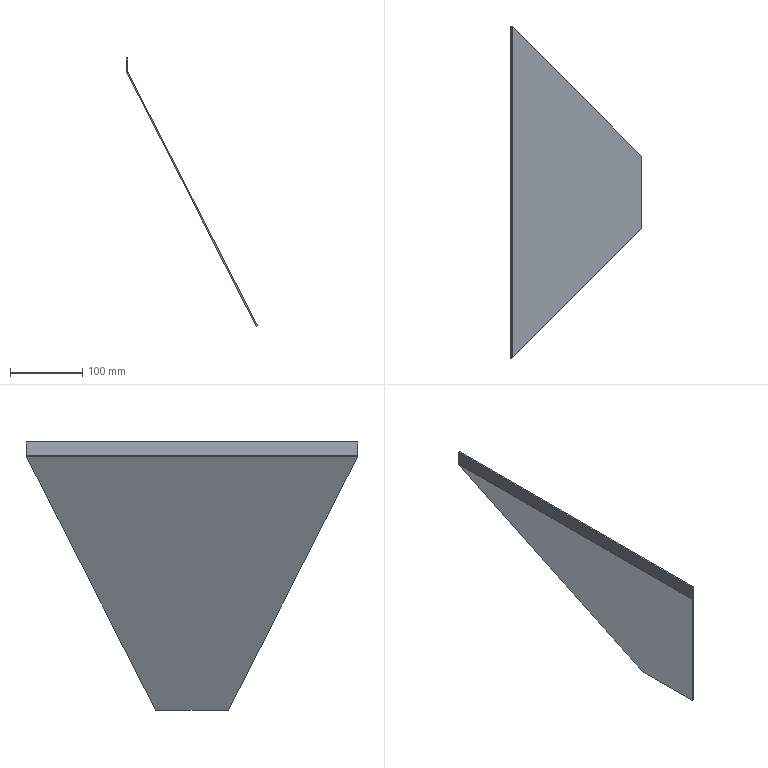Part | SolidWorks | features ICE 3, Blend 1, FlatPattern 1, SheetMetal 1, Shell 1, SolidToSheetMetal 1 | 1 solid | 14 faces | box 180.781 x 458 x 370 mm | volume 237222 mm3 | plane 10 | spline 2 | cylinder 2 | commonest cylinder face diameters 2 x1 6 x1
STEP:
#1=CARTESIAN_POINT('',(-227.,-229.,0.7226));
#2=VERTEX_POINT('',#1);
#3=CARTESIAN_POINT('',(-229.,-229.,0.7226));
#4=VERTEX_POINT('',#3);
#5=CARTESIAN_POINT('',(-229.,-229.,0.7226));
#6=DIRECTION('',(-1.,0.,0.));
#7=VECTOR('',#6,1000.);
#8=LINE('',#5,#7);
#9=EDGE_CURVE('',#2,#4,#8,.T.);
#10=ORIENTED_EDGE('',*,*,#9,.F.);
#11=CARTESIAN_POINT('',(-227.,-229.,20.));
#12=VERTEX_POINT('',#11);
#13=CARTESIAN_POINT('',(-227.,-229.,20.));
#14=DIRECTION('',(0.,0.,-1.));
#15=VECTOR('',#14,1000.);
#16=LINE('',#13,#15);
#17=EDGE_CURVE('',#12,#2,#16,.T.);
#18=ORIENTED_EDGE('',*,*,#17,.F.);
#19=CARTESIAN_POINT('',(-229.,-229.,20.));
#20=VERTEX_POINT('',#19);
#21=CARTESIAN_POINT('',(-229.,-229.,20.));
#22=DIRECTION('',(-1.,0.,0.));
#23=VECTOR('',#22,1000.);
#24=LINE('',#21,#23);
#25=EDGE_CURVE('',#12,#20,#24,.T.);
#26=ORIENTED_EDGE('',*,*,#25,.T.);
#27=CARTESIAN_POINT('',(-229.,-229.,20.));
#28=DIRECTION('',(0.,0.,-1.));
#29=VECTOR('',#28,1000.);
#30=LINE('',#27,#29);
#31=EDGE_CURVE('',#20,#4,#30,.T.);
#32=ORIENTED_EDGE('',*,*,#31,.T.);
#33=EDGE_LOOP('',(#10,#18,#26,#32));
#34=FACE_OUTER_BOUND('',#33,.T.);
#35=CARTESIAN_POINT('',(-229.,-229.,20.));
#36=DIRECTION('',(0.,-1.,0.));
#37=DIRECTION('',(0.,0.,-1.));
#38=AXIS2_PLACEMENT_3D('',#35,#36,#37);
#39=PLANE('',#38);
#40=ADVANCED_FACE('',(#34),#39,.T.);
#41=ORIENTED_EDGE('',*,*,#25,.F.);
#42=CARTESIAN_POINT('',(-227.,229.,20.));
#43=VERTEX_POINT('',#42);
#44=CARTESIAN_POINT('',(-227.,229.,20.));
#45=DIRECTION('',(0.,-1.,0.));
#46=VECTOR('',#45,1000.);
#47=LINE('',#44,#46);
#48=EDGE_CURVE('',#43,#12,#47,.T.);
#49=ORIENTED_EDGE('',*,*,#48,.F.);
#50=CARTESIAN_POINT('',(-229.,229.,20.));
#51=VERTEX_POINT('',#50);
#52=CARTESIAN_POINT('',(-229.,229.,20.));
#53=DIRECTION('',(-1.,0.,0.));
#54=VECTOR('',#53,1000.);
#55=LINE('',#52,#54);
#56=EDGE_CURVE('',#43,#51,#55,.T.);
#57=ORIENTED_EDGE('',*,*,#56,.T.);
#58=CARTESIAN_POINT('',(-229.,229.,20.));
#59=DIRECTION('',(0.,-1.,0.));
#60=VECTOR('',#59,1000.);
#61=LINE('',#58,#60);
#62=EDGE_CURVE('',#51,#20,#61,.T.);
#63=ORIENTED_EDGE('',*,*,#62,.T.);
#64=EDGE_LOOP('',(#41,#49,#57,#63));
#65=FACE_OUTER_BOUND('',#64,.T.);
#66=CARTESIAN_POINT('',(-229.,229.,20.));
#67=DIRECTION('',(0.,0.,1.));
#68=DIRECTION('',(0.,-1.,0.));
#69=AXIS2_PLACEMENT_3D('',#66,#67,#68);
#70=PLANE('',#69);
#71=ADVANCED_FACE('',(#65),#70,.T.);
#72=ORIENTED_EDGE('',*,*,#56,.F.);
#73=CARTESIAN_POINT('',(-227.,229.,0.7226));
#74=VERTEX_POINT('',#73);
#75=CARTESIAN_POINT('',(-227.,229.,20.));
#76=DIRECTION('',(0.,0.,-1.));
#77=VECTOR('',#76,1000.);
#78=LINE('',#75,#77);
#79=EDGE_CURVE('',#43,#74,#78,.T.);
#80=ORIENTED_EDGE('',*,*,#79,.T.);
#81=CARTESIAN_POINT('',(-229.,229.,0.7226));
#82=VERTEX_POINT('',#81);
#83=CARTESIAN_POINT('',(-229.,229.,0.7226));
#84=DIRECTION('',(-1.,0.,0.));
#85=VECTOR('',#84,1000.);
#86=LINE('',#83,#85);
#87=EDGE_CURVE('',#74,#82,#86,.T.);
#88=ORIENTED_EDGE('',*,*,#87,.T.);
#89=CARTESIAN_POINT('',(-229.,229.,20.));
#90=DIRECTION('',(0.,0.,-1.));
#91=VECTOR('',#90,1000.);
#92=LINE('',#89,#91);
#93=EDGE_CURVE('',#51,#82,#92,.T.);
#94=ORIENTED_EDGE('',*,*,#93,.F.);
#95=EDGE_LOOP('',(#72,#80,#88,#94));
#96=FACE_OUTER_BOUND('',#95,.T.);
#97=CARTESIAN_POINT('',(-229.,229.,20.));
#98=DIRECTION('',(0.,-1.,0.));
#99=DIRECTION('',(0.,0.,-1.));
#100=AXIS2_PLACEMENT_3D('',#97,#98,#99);
#101=PLANE('',#100);
#102=ADVANCED_FACE('',(#96),#101,.F.);
#103=ORIENTED_EDGE('',*,*,#87,.F.);
#104=CARTESIAN_POINT('',(-226.89,228.671,0.2673));
#105=VERTEX_POINT('',#104);
#106=CARTESIAN_POINT('',(-227.,229.,0.7226));
#107=CARTESIAN_POINT('',(-227.,229.,0.5636));
#108=CARTESIAN_POINT('',(-226.963,228.888,0.4089));
#109=CARTESIAN_POINT('',(-226.89,228.671,0.2673));
#110=(BOUNDED_CURVE()B_SPLINE_CURVE(3,(#106,#107,#108,#109),.UNSPECIFIED.,.F.,.T.)B_SPLINE_CURVE_WITH_KNOTS((4,4),(0.,0.4727),.UNSPECIFIED.)CURVE()GEOMETRIC_REPRESENTATION_ITEM()RATIONAL_B_SPLINE_CURVE((1.,0.9815,0.9815,1.))REPRESENTATION_ITEM(''));
#111=EDGE_CURVE('',#74,#105,#110,.T.);
#112=ORIENTED_EDGE('',*,*,#111,.T.);
#113=CARTESIAN_POINT('',(-228.671,228.671,-0.6434));
#114=VERTEX_POINT('',#113);
#115=CARTESIAN_POINT('',(-228.671,228.671,-0.6434));
#116=DIRECTION('',(-0.8903,0.,-0.4553));
#117=VECTOR('',#116,1000.);
#118=LINE('',#115,#117);
#119=EDGE_CURVE('',#105,#114,#118,.T.);
#120=ORIENTED_EDGE('',*,*,#119,.T.);
#121=CARTESIAN_POINT('',(-229.,229.,0.7226));
#122=CARTESIAN_POINT('',(-229.,229.,0.2454));
#123=CARTESIAN_POINT('',(-228.888,228.888,-0.2185));
#124=CARTESIAN_POINT('',(-228.671,228.671,-0.6434));
#125=(BOUNDED_CURVE()B_SPLINE_CURVE(3,(#121,#122,#123,#124),.UNSPECIFIED.,.F.,.F.)B_SPLINE_CURVE_WITH_KNOTS((4,4),(0.,0.4727),.UNSPECIFIED.)CURVE()GEOMETRIC_REPRESENTATION_ITEM()RATIONAL_B_SPLINE_CURVE((1.,0.9815,0.9815,1.))REPRESENTATION_ITEM(''));
#126=EDGE_CURVE('',#82,#114,#125,.T.);
#127=ORIENTED_EDGE('',*,*,#126,.F.);
#128=EDGE_LOOP('',(#103,#112,#120,#127));
#129=FACE_OUTER_BOUND('',#128,.T.);
#130=CARTESIAN_POINT('',(-229.,229.,0.7226));
#131=CARTESIAN_POINT('',(-228.333,229.,0.7226));
#132=CARTESIAN_POINT('',(-227.667,229.,0.7226));
#133=CARTESIAN_POINT('',(-227.,229.,0.7226));
#134=CARTESIAN_POINT('',(-229.,229.,-5.277));
#135=CARTESIAN_POINT('',(-228.333,229.,-3.944));
#136=CARTESIAN_POINT('',(-227.667,229.,-2.611));
#137=CARTESIAN_POINT('',(-227.,229.,-1.277));
#138=CARTESIAN_POINT('',(-223.,223.,-5.277));
#139=CARTESIAN_POINT('',(-223.667,223.,-3.944));
#140=CARTESIAN_POINT('',(-224.333,223.,-2.611));
#141=CARTESIAN_POINT('',(-225.,223.,-1.277));
#142=CARTESIAN_POINT('',(-223.,223.,0.7226));
#143=CARTESIAN_POINT('',(-223.667,223.,0.7226));
#144=CARTESIAN_POINT('',(-224.333,223.,0.7226));
#145=CARTESIAN_POINT('',(-225.,223.,0.7226));
#146=CARTESIAN_POINT('',(-223.,223.,6.723));
#147=CARTESIAN_POINT('',(-223.667,223.,5.389));
#148=CARTESIAN_POINT('',(-224.333,223.,4.056));
#149=CARTESIAN_POINT('',(-225.,223.,2.723));
#150=CARTESIAN_POINT('',(-229.,229.,6.723));
#151=CARTESIAN_POINT('',(-228.333,229.,5.389));
#152=CARTESIAN_POINT('',(-227.667,229.,4.056));
#153=CARTESIAN_POINT('',(-227.,229.,2.723));
#154=CARTESIAN_POINT('',(-229.,229.,0.7226));
#155=CARTESIAN_POINT('',(-228.333,229.,0.7226));
#156=CARTESIAN_POINT('',(-227.667,229.,0.7226));
#157=CARTESIAN_POINT('',(-227.,229.,0.7226));
#158=(BOUNDED_SURFACE()B_SPLINE_SURFACE(3,3,((#130,#131,#132,#133),(#134,#135,#136,#137),(#138,#139,#140,#141),(#142,#143,#144,#145),(#146,#147,#148,#149),(#150,#151,#152,#153),(#154,#155,#156,#157)),.UNSPECIFIED.,.T.,.F.,.T.)B_SPLINE_SURFACE_WITH_KNOTS((4,3,4),(4,4),(0.,0.5,1.),(0.,1.),.UNSPECIFIED.)GEOMETRIC_REPRESENTATION_ITEM()RATIONAL_B_SPLINE_SURFACE(((1.,1.,1.,1.),(0.3333,0.3333,0.3333,0.3333),(0.3333,0.3333,0.3333,0.3333),(1.,1.,1.,1.),(0.3333,0.3333,0.3333,0.3333),(0.3333,0.3333,0.3333,0.3333),(1.,1.,1.,1.)))REPRESENTATION_ITEM('')SURFACE());
#159=ADVANCED_FACE('',(#129),#158,.F.);
#160=ORIENTED_EDGE('',*,*,#119,.F.);
#161=CARTESIAN_POINT('',(-48.219,50.,-349.089));
#162=VERTEX_POINT('',#161);
#163=CARTESIAN_POINT('',(-227.219,229.,0.9107));
#164=DIRECTION('',(0.4144,-0.4144,-0.8103));
#165=VECTOR('',#164,1000.);
#166=LINE('',#163,#165);
#167=EDGE_CURVE('',#105,#162,#166,.T.);
#168=ORIENTED_EDGE('',*,*,#167,.T.);
#169=CARTESIAN_POINT('',(-50.,50.,-350.));
#170=VERTEX_POINT('',#169);
#171=CARTESIAN_POINT('',(-48.219,50.,-349.089));
#172=CARTESIAN_POINT('',(-48.813,50.,-349.393));
#173=CARTESIAN_POINT('',(-49.406,50.,-349.696));
#174=CARTESIAN_POINT('',(-50.,50.,-350.));
#175=B_SPLINE_CURVE_WITH_KNOTS('',3,(#171,#172,#173,#174),.UNSPECIFIED.,.F.,.F.,(4,4),(0.,1.),.UNSPECIFIED.);
#176=EDGE_CURVE('',#162,#170,#175,.T.);
#177=ORIENTED_EDGE('',*,*,#176,.T.);
#178=CARTESIAN_POINT('',(-229.,229.,0.));
#179=DIRECTION('',(0.4144,-0.4144,-0.8103));
#180=VECTOR('',#179,1000.);
#181=LINE('',#178,#180);
#182=EDGE_CURVE('',#114,#170,#181,.T.);
#183=ORIENTED_EDGE('',*,*,#182,.F.);
#184=EDGE_LOOP('',(#160,#168,#177,#183));
#185=FACE_OUTER_BOUND('',#184,.T.);
#186=CARTESIAN_POINT('',(-229.,229.,0.));
#187=DIRECTION('',(0.1887,0.9101,-0.3689));
#188=DIRECTION('',(0.4144,-0.4144,-0.8103));
#189=AXIS2_PLACEMENT_3D('',#186,#187,#188);
#190=PLANE('',#189);
#191=ADVANCED_FACE('',(#185),#190,.T.);
#192=ORIENTED_EDGE('',*,*,#176,.F.);
#193=CARTESIAN_POINT('',(-48.219,-50.,-349.089));
#194=VERTEX_POINT('',#193);
#195=CARTESIAN_POINT('',(-48.219,50.,-349.089));
#196=CARTESIAN_POINT('',(-48.219,16.667,-349.089));
#197=CARTESIAN_POINT('',(-48.219,-16.667,-349.089));
#198=CARTESIAN_POINT('',(-48.219,-50.,-349.089));
#199=B_SPLINE_CURVE_WITH_KNOTS('',3,(#195,#196,#197,#198),.UNSPECIFIED.,.F.,.F.,(4,4),(0.,1.),.UNSPECIFIED.);
#200=EDGE_CURVE('',#162,#194,#199,.T.);
#201=ORIENTED_EDGE('',*,*,#200,.T.);
#202=CARTESIAN_POINT('',(-50.,-50.,-350.));
#203=VERTEX_POINT('',#202);
#204=CARTESIAN_POINT('',(-48.219,-50.,-349.089));
#205=CARTESIAN_POINT('',(-48.813,-50.,-349.393));
#206=CARTESIAN_POINT('',(-49.406,-50.,-349.696));
#207=CARTESIAN_POINT('',(-50.,-50.,-350.));
#208=B_SPLINE_CURVE_WITH_KNOTS('',3,(#204,#205,#206,#207),.UNSPECIFIED.,.F.,.F.,(4,4),(0.,1.),.UNSPECIFIED.);
#209=EDGE_CURVE('',#194,#203,#208,.T.);
#210=ORIENTED_EDGE('',*,*,#209,.T.);
#211=CARTESIAN_POINT('',(-50.,50.,-350.));
#212=DIRECTION('',(0.,-1.,0.));
#213=VECTOR('',#212,1000.);
#214=LINE('',#211,#213);
#215=EDGE_CURVE('',#170,#203,#214,.T.);
#216=ORIENTED_EDGE('',*,*,#215,.F.);
#217=EDGE_LOOP('',(#192,#201,#210,#216));
#218=FACE_OUTER_BOUND('',#217,.T.);
#219=CARTESIAN_POINT('',(-50.,50.,-350.));
#220=DIRECTION('',(0.4553,0.,-0.8903));
#221=DIRECTION('',(0.,-1.,0.));
#222=AXIS2_PLACEMENT_3D('',#219,#220,#221);
#223=PLANE('',#222);
#224=ADVANCED_FACE('',(#218),#223,.T.);
#225=ORIENTED_EDGE('',*,*,#209,.F.);
#226=CARTESIAN_POINT('',(-226.89,-228.671,0.2673));
#227=VERTEX_POINT('',#226);
#228=CARTESIAN_POINT('',(-227.219,-229.,0.9107));
#229=DIRECTION('',(0.4144,0.4144,-0.8103));
#230=VECTOR('',#229,1000.);
#231=LINE('',#228,#230);
#232=EDGE_CURVE('',#227,#194,#231,.T.);
#233=ORIENTED_EDGE('',*,*,#232,.F.);
#234=CARTESIAN_POINT('',(-228.671,-228.671,-0.6434));
#235=VERTEX_POINT('',#234);
#236=CARTESIAN_POINT('',(-228.671,-228.671,-0.6434));
#237=DIRECTION('',(-0.8903,0.,-0.4553));
#238=VECTOR('',#237,1000.);
#239=LINE('',#236,#238);
#240=EDGE_CURVE('',#227,#235,#239,.T.);
#241=ORIENTED_EDGE('',*,*,#240,.T.);
#242=CARTESIAN_POINT('',(-229.,-229.,0.));
#243=DIRECTION('',(0.4144,0.4144,-0.8103));
#244=VECTOR('',#243,1000.);
#245=LINE('',#242,#244);
#246=EDGE_CURVE('',#235,#203,#245,.T.);
#247=ORIENTED_EDGE('',*,*,#246,.T.);
#248=EDGE_LOOP('',(#225,#233,#241,#247));
#249=FACE_OUTER_BOUND('',#248,.T.);
#250=CARTESIAN_POINT('',(-229.,-229.,0.));
#251=DIRECTION('',(-0.1887,0.9101,0.3689));
#252=DIRECTION('',(0.4144,0.4144,-0.8103));
#253=AXIS2_PLACEMENT_3D('',#250,#251,#252);
#254=PLANE('',#253);
#255=ADVANCED_FACE('',(#249),#254,.F.);
#256=CARTESIAN_POINT('',(-226.89,-228.671,0.2673));
#257=CARTESIAN_POINT('',(-226.963,-228.888,0.4089));
#258=CARTESIAN_POINT('',(-227.,-229.,0.5636));
#259=CARTESIAN_POINT('',(-227.,-229.,0.7226));
#260=(BOUNDED_CURVE()B_SPLINE_CURVE(3,(#256,#257,#258,#259),.UNSPECIFIED.,.F.,.F.)B_SPLINE_CURVE_WITH_KNOTS((4,4),(2.669,3.142),.UNSPECIFIED.)CURVE()GEOMETRIC_REPRESENTATION_ITEM()RATIONAL_B_SPLINE_CURVE((1.,0.9815,0.9815,1.))REPRESENTATION_ITEM(''));
#261=EDGE_CURVE('',#227,#2,#260,.T.);
#262=ORIENTED_EDGE('',*,*,#261,.T.);
#263=ORIENTED_EDGE('',*,*,#9,.T.);
#264=CARTESIAN_POINT('',(-228.671,-228.671,-0.6434));
#265=CARTESIAN_POINT('',(-228.888,-228.888,-0.2185));
#266=CARTESIAN_POINT('',(-229.,-229.,0.2454));
#267=CARTESIAN_POINT('',(-229.,-229.,0.7226));
#268=(BOUNDED_CURVE()B_SPLINE_CURVE(3,(#264,#265,#266,#267),.UNSPECIFIED.,.F.,.T.)B_SPLINE_CURVE_WITH_KNOTS((4,4),(2.669,3.142),.UNSPECIFIED.)CURVE()GEOMETRIC_REPRESENTATION_ITEM()RATIONAL_B_SPLINE_CURVE((1.,0.9815,0.9815,1.))REPRESENTATION_ITEM(''));
#269=EDGE_CURVE('',#235,#4,#268,.T.);
#270=ORIENTED_EDGE('',*,*,#269,.F.);
#271=ORIENTED_EDGE('',*,*,#240,.F.);
#272=EDGE_LOOP('',(#262,#263,#270,#271));
#273=FACE_OUTER_BOUND('',#272,.T.);
#274=CARTESIAN_POINT('',(-223.,-223.,0.7226));
#275=CARTESIAN_POINT('',(-223.667,-223.,0.7226));
#276=CARTESIAN_POINT('',(-224.333,-223.,0.7226));
#277=CARTESIAN_POINT('',(-225.,-223.,0.7226));
#278=CARTESIAN_POINT('',(-223.,-223.,-5.277));
#279=CARTESIAN_POINT('',(-223.667,-223.,-3.944));
#280=CARTESIAN_POINT('',(-224.333,-223.,-2.611));
#281=CARTESIAN_POINT('',(-225.,-223.,-1.277));
#282=CARTESIAN_POINT('',(-229.,-229.,-5.277));
#283=CARTESIAN_POINT('',(-228.333,-229.,-3.944));
#284=CARTESIAN_POINT('',(-227.667,-229.,-2.611));
#285=CARTESIAN_POINT('',(-227.,-229.,-1.277));
#286=CARTESIAN_POINT('',(-229.,-229.,0.7226));
#287=CARTESIAN_POINT('',(-228.333,-229.,0.7226));
#288=CARTESIAN_POINT('',(-227.667,-229.,0.7226));
#289=CARTESIAN_POINT('',(-227.,-229.,0.7226));
#290=CARTESIAN_POINT('',(-229.,-229.,6.723));
#291=CARTESIAN_POINT('',(-228.333,-229.,5.389));
#292=CARTESIAN_POINT('',(-227.667,-229.,4.056));
#293=CARTESIAN_POINT('',(-227.,-229.,2.723));
#294=CARTESIAN_POINT('',(-223.,-223.,6.723));
#295=CARTESIAN_POINT('',(-223.667,-223.,5.389));
#296=CARTESIAN_POINT('',(-224.333,-223.,4.056));
#297=CARTESIAN_POINT('',(-225.,-223.,2.723));
#298=CARTESIAN_POINT('',(-223.,-223.,0.7226));
#299=CARTESIAN_POINT('',(-223.667,-223.,0.7226));
#300=CARTESIAN_POINT('',(-224.333,-223.,0.7226));
#301=CARTESIAN_POINT('',(-225.,-223.,0.7226));
#302=(BOUNDED_SURFACE()B_SPLINE_SURFACE(3,3,((#274,#275,#276,#277),(#278,#279,#280,#281),(#282,#283,#284,#285),(#286,#287,#288,#289),(#290,#291,#292,#293),(#294,#295,#296,#297),(#298,#299,#300,#301)),.UNSPECIFIED.,.T.,.F.,.F.)B_SPLINE_SURFACE_WITH_KNOTS((4,3,4),(4,4),(0.,0.5,1.),(0.,1.),.UNSPECIFIED.)GEOMETRIC_REPRESENTATION_ITEM()RATIONAL_B_SPLINE_SURFACE(((1.,1.,1.,1.),(0.3333,0.3333,0.3333,0.3333),(0.3333,0.3333,0.3333,0.3333),(1.,1.,1.,1.),(0.3333,0.3333,0.3333,0.3333),(0.3333,0.3333,0.3333,0.3333),(1.,1.,1.,1.)))REPRESENTATION_ITEM('')SURFACE());
#303=ADVANCED_FACE('',(#273),#302,.F.);
#304=ORIENTED_EDGE('',*,*,#246,.F.);
#305=CARTESIAN_POINT('',(-228.671,229.,-0.6434));
#306=DIRECTION('',(0.,1.,0.));
#307=VECTOR('',#306,1000.);
#308=LINE('',#305,#307);
#309=EDGE_CURVE('',#235,#114,#308,.T.);
#310=ORIENTED_EDGE('',*,*,#309,.T.);
#311=ORIENTED_EDGE('',*,*,#182,.T.);
#312=ORIENTED_EDGE('',*,*,#215,.T.);
#313=EDGE_LOOP('',(#304,#310,#311,#312));
#314=FACE_OUTER_BOUND('',#313,.T.);
#315=CARTESIAN_POINT('',(-181.521,0.,-92.835));
#316=DIRECTION('',(-0.8903,0.,-0.4553));
#317=DIRECTION('',(-0.4553,0.,0.8903));
#318=AXIS2_PLACEMENT_3D('',#315,#316,#317);
#319=PLANE('',#318);
#320=ADVANCED_FACE('',(#314),#319,.T.);
#321=ORIENTED_EDGE('',*,*,#93,.T.);
#322=CARTESIAN_POINT('',(-229.,-229.,0.7226));
#323=DIRECTION('',(0.,-1.,0.));
#324=VECTOR('',#323,1000.);
#325=LINE('',#322,#324);
#326=EDGE_CURVE('',#82,#4,#325,.T.);
#327=ORIENTED_EDGE('',*,*,#326,.T.);
#328=ORIENTED_EDGE('',*,*,#31,.F.);
#329=ORIENTED_EDGE('',*,*,#62,.F.);
#330=EDGE_LOOP('',(#321,#327,#328,#329));
#331=FACE_OUTER_BOUND('',#330,.T.);
#332=CARTESIAN_POINT('',(-229.,229.,20.));
#333=DIRECTION('',(1.,0.,0.));
#334=DIRECTION('',(0.,1.,0.));
#335=AXIS2_PLACEMENT_3D('',#332,#333,#334);
#336=PLANE('',#335);
#337=ADVANCED_FACE('',(#331),#336,.F.);
#338=ORIENTED_EDGE('',*,*,#126,.T.);
#339=ORIENTED_EDGE('',*,*,#309,.F.);
#340=ORIENTED_EDGE('',*,*,#269,.T.);
#341=ORIENTED_EDGE('',*,*,#326,.F.);
#342=EDGE_LOOP('',(#338,#339,#340,#341));
#343=FACE_OUTER_BOUND('',#342,.T.);
#344=CARTESIAN_POINT('',(-226.,229.,0.7226));
#345=DIRECTION('',(0.,1.,0.));
#346=DIRECTION('',(0.,0.,1.));
#347=AXIS2_PLACEMENT_3D('',#344,#345,#346);
#348=CYLINDRICAL_SURFACE('',#347,3.);
#349=ADVANCED_FACE('',(#343),#348,.T.);
#350=ORIENTED_EDGE('',*,*,#232,.T.);
#351=ORIENTED_EDGE('',*,*,#200,.F.);
#352=ORIENTED_EDGE('',*,*,#167,.F.);
#353=CARTESIAN_POINT('',(-226.89,0.,0.2673));
#354=DIRECTION('',(0.,1.,0.));
#355=VECTOR('',#354,1000.);
#356=LINE('',#353,#355);
#357=EDGE_CURVE('',#227,#105,#356,.T.);
#358=ORIENTED_EDGE('',*,*,#357,.F.);
#359=EDGE_LOOP('',(#350,#351,#352,#358));
#360=FACE_OUTER_BOUND('',#359,.T.);
#361=CARTESIAN_POINT('',(-179.741,0.,-91.925));
#362=DIRECTION('',(-0.8903,0.,-0.4553));
#363=DIRECTION('',(-0.4553,0.,0.8903));
#364=AXIS2_PLACEMENT_3D('',#361,#362,#363);
#365=PLANE('',#364);
#366=ADVANCED_FACE('',(#360),#365,.F.);
#367=ORIENTED_EDGE('',*,*,#79,.F.);
#368=ORIENTED_EDGE('',*,*,#48,.T.);
#369=ORIENTED_EDGE('',*,*,#17,.T.);
#370=CARTESIAN_POINT('',(-227.,229.,0.7226));
#371=DIRECTION('',(0.,-1.,0.));
#372=VECTOR('',#371,1000.);
#373=LINE('',#370,#372);
#374=EDGE_CURVE('',#74,#2,#373,.T.);
#375=ORIENTED_EDGE('',*,*,#374,.F.);
#376=EDGE_LOOP('',(#367,#368,#369,#375));
#377=FACE_OUTER_BOUND('',#376,.T.);
#378=CARTESIAN_POINT('',(-227.,229.,20.));
#379=DIRECTION('',(1.,0.,0.));
#380=DIRECTION('',(0.,1.,0.));
#381=AXIS2_PLACEMENT_3D('',#378,#379,#380);
#382=PLANE('',#381);
#383=ADVANCED_FACE('',(#377),#382,.T.);
#384=ORIENTED_EDGE('',*,*,#111,.F.);
#385=ORIENTED_EDGE('',*,*,#374,.T.);
#386=ORIENTED_EDGE('',*,*,#261,.F.);
#387=ORIENTED_EDGE('',*,*,#357,.T.);
#388=EDGE_LOOP('',(#384,#385,#386,#387));
#389=FACE_OUTER_BOUND('',#388,.T.);
#390=CARTESIAN_POINT('',(-226.,229.,0.7226));
#391=DIRECTION('',(0.,1.,0.));
#392=DIRECTION('',(0.,0.,1.));
#393=AXIS2_PLACEMENT_3D('',#390,#391,#392);
#394=CYLINDRICAL_SURFACE('',#393,1.);
#395=ADVANCED_FACE('',(#389),#394,.F.);
#396=CLOSED_SHELL('',(#40,#71,#102,#159,#191,#224,#255,#303,#320,#337,#349,#366,#383,#395));
#397=MANIFOLD_SOLID_BREP('',#396);
#398=CARTESIAN_POINT('',(0.,0.,0.));
#399=DIRECTION('',(0.,0.,1.));
#400=DIRECTION('',(1.,0.,0.));
#401=AXIS2_PLACEMENT_3D('',#398,#399,#400);
#402=(LENGTH_UNIT()NAMED_UNIT(*)SI_UNIT(.MILLI.,.METRE.));
#403=UNCERTAINTY_MEASURE_WITH_UNIT(LENGTH_MEASURE(0.00001),#402,'','');
#404=(NAMED_UNIT(*)PLANE_ANGLE_UNIT()SI_UNIT($,.RADIAN.));
#405=(NAMED_UNIT(*)SI_UNIT($,.STERADIAN.)SOLID_ANGLE_UNIT());
#406=(GEOMETRIC_REPRESENTATION_CONTEXT(3)GLOBAL_UNCERTAINTY_ASSIGNED_CONTEXT((#403))GLOBAL_UNIT_ASSIGNED_CONTEXT((#402,#404,#405))REPRESENTATION_CONTEXT('',''));
#407=ADVANCED_BREP_SHAPE_REPRESENTATION('',(#397,#401),#406);